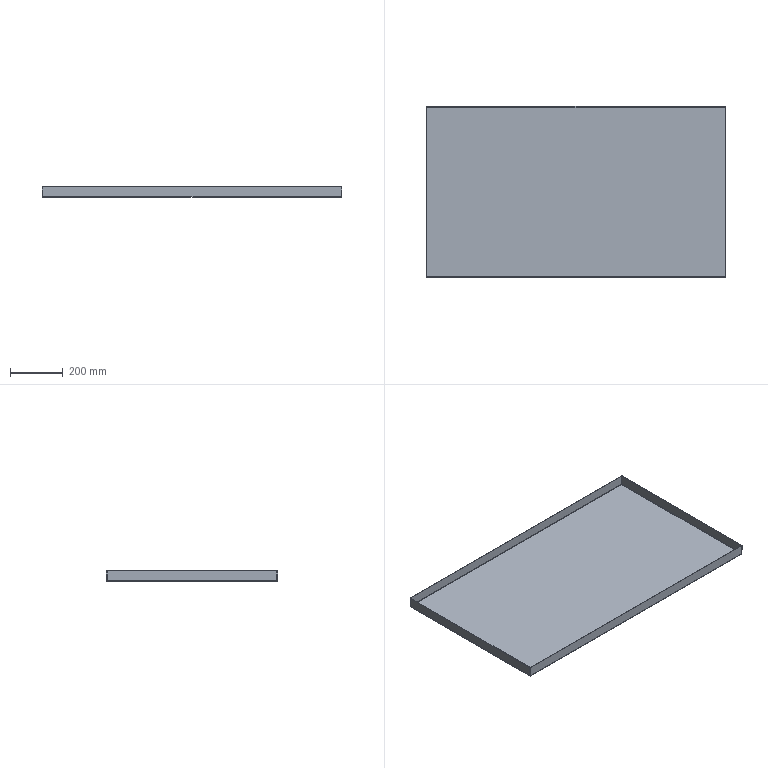Part | SolidWorks | features EdgeFlange 1, FlatPattern 1, SMBaseFlange 1, SheetMetal 1 | 1 solid | 38 faces | box 1140 x 650 x 40 mm | volume 1747070 mm3 | plane 22 | spline 8 | cylinder 8 | commonest cylinder face diameters 1.473 x4 5.473 x4
STEP:
#1=CARTESIAN_POINT('',(567.263,322.263,-2.));
#2=VERTEX_POINT('',#1);
#3=CARTESIAN_POINT('',(567.263,-322.263,-2.));
#4=VERTEX_POINT('',#3);
#5=CARTESIAN_POINT('',(567.263,322.293,-2.));
#6=DIRECTION('',(0.,-1.,0.));
#7=VECTOR('',#6,1000.);
#8=LINE('',#5,#7);
#9=EDGE_CURVE('',#2,#4,#8,.T.);
#10=ORIENTED_EDGE('',*,*,#9,.T.);
#11=CARTESIAN_POINT('',(-567.263,-322.263,-2.));
#12=VERTEX_POINT('',#11);
#13=CARTESIAN_POINT('',(567.293,-322.263,-2.));
#14=DIRECTION('',(-1.,0.,0.));
#15=VECTOR('',#14,1000.);
#16=LINE('',#13,#15);
#17=EDGE_CURVE('',#4,#12,#16,.T.);
#18=ORIENTED_EDGE('',*,*,#17,.T.);
#19=CARTESIAN_POINT('',(-567.263,322.263,-2.));
#20=VERTEX_POINT('',#19);
#21=CARTESIAN_POINT('',(-567.263,-322.293,-2.));
#22=DIRECTION('',(0.,1.,0.));
#23=VECTOR('',#22,1000.);
#24=LINE('',#21,#23);
#25=EDGE_CURVE('',#12,#20,#24,.T.);
#26=ORIENTED_EDGE('',*,*,#25,.T.);
#27=CARTESIAN_POINT('',(-567.293,322.263,-2.));
#28=DIRECTION('',(1.,0.,0.));
#29=VECTOR('',#28,1000.);
#30=LINE('',#27,#29);
#31=EDGE_CURVE('',#20,#2,#30,.T.);
#32=ORIENTED_EDGE('',*,*,#31,.T.);
#33=EDGE_LOOP('',(#10,#18,#26,#32));
#34=FACE_OUTER_BOUND('',#33,.T.);
#35=CARTESIAN_POINT('',(0.,0.,-2.));
#36=DIRECTION('',(0.,0.,-1.));
#37=DIRECTION('',(-1.,0.,0.));
#38=AXIS2_PLACEMENT_3D('',#35,#36,#37);
#39=PLANE('',#38);
#40=ADVANCED_FACE('',(#34),#39,.T.);
#41=CARTESIAN_POINT('',(567.263,-322.263,0.));
#42=VERTEX_POINT('',#41);
#43=CARTESIAN_POINT('',(-567.263,-322.263,0.));
#44=VERTEX_POINT('',#43);
#45=CARTESIAN_POINT('',(567.293,-322.263,0.));
#46=DIRECTION('',(-1.,0.,0.));
#47=VECTOR('',#46,1000.);
#48=LINE('',#45,#47);
#49=EDGE_CURVE('',#42,#44,#48,.T.);
#50=ORIENTED_EDGE('',*,*,#49,.F.);
#51=CARTESIAN_POINT('',(567.263,322.263,0.));
#52=VERTEX_POINT('',#51);
#53=CARTESIAN_POINT('',(567.263,322.293,0.));
#54=DIRECTION('',(0.,-1.,0.));
#55=VECTOR('',#54,1000.);
#56=LINE('',#53,#55);
#57=EDGE_CURVE('',#52,#42,#56,.T.);
#58=ORIENTED_EDGE('',*,*,#57,.F.);
#59=CARTESIAN_POINT('',(-567.263,322.263,0.));
#60=VERTEX_POINT('',#59);
#61=CARTESIAN_POINT('',(-567.293,322.263,0.));
#62=DIRECTION('',(1.,0.,0.));
#63=VECTOR('',#62,1000.);
#64=LINE('',#61,#63);
#65=EDGE_CURVE('',#60,#52,#64,.T.);
#66=ORIENTED_EDGE('',*,*,#65,.F.);
#67=CARTESIAN_POINT('',(-567.263,-322.293,0.));
#68=DIRECTION('',(0.,1.,0.));
#69=VECTOR('',#68,1000.);
#70=LINE('',#67,#69);
#71=EDGE_CURVE('',#44,#60,#70,.T.);
#72=ORIENTED_EDGE('',*,*,#71,.F.);
#73=EDGE_LOOP('',(#50,#58,#66,#72));
#74=FACE_OUTER_BOUND('',#73,.T.);
#75=CARTESIAN_POINT('',(0.,0.,0.));
#76=DIRECTION('',(0.,0.,-1.));
#77=DIRECTION('',(-1.,0.,0.));
#78=AXIS2_PLACEMENT_3D('',#75,#76,#77);
#79=PLANE('',#78);
#80=ADVANCED_FACE('',(#74),#79,.F.);
#81=CARTESIAN_POINT('',(567.293,325.,0.7366));
#82=VERTEX_POINT('',#81);
#83=CARTESIAN_POINT('',(567.293,323.,0.7366));
#84=VERTEX_POINT('',#83);
#85=CARTESIAN_POINT('',(567.293,323.,0.7366));
#86=DIRECTION('',(0.,-1.,0.));
#87=VECTOR('',#86,1000.);
#88=LINE('',#85,#87);
#89=EDGE_CURVE('',#82,#84,#88,.T.);
#90=ORIENTED_EDGE('',*,*,#89,.T.);
#91=CARTESIAN_POINT('',(567.263,322.263,0.));
#92=CARTESIAN_POINT('',(567.268,322.456,0.));
#93=CARTESIAN_POINT('',(567.273,322.648,0.07939));
#94=CARTESIAN_POINT('',(567.283,322.921,0.3521));
#95=CARTESIAN_POINT('',(567.288,323.,0.5438));
#96=CARTESIAN_POINT('',(567.293,323.,0.7366));
#97=B_SPLINE_CURVE_WITH_KNOTS('',3,(#91,#92,#93,#94,#95,#96),.UNSPECIFIED.,.F.,.F.,(4,2,4),(0.,0.5,1.),.UNSPECIFIED.);
#98=EDGE_CURVE('',#52,#84,#97,.T.);
#99=ORIENTED_EDGE('',*,*,#98,.F.);
#100=CARTESIAN_POINT('',(567.263,322.263,0.));
#101=DIRECTION('',(0.,0.,-1.));
#102=VECTOR('',#101,1000.);
#103=LINE('',#100,#102);
#104=EDGE_CURVE('',#52,#2,#103,.T.);
#105=ORIENTED_EDGE('',*,*,#104,.T.);
#106=CARTESIAN_POINT('',(567.263,322.263,-2.));
#107=CARTESIAN_POINT('',(567.266,322.622,-2.));
#108=CARTESIAN_POINT('',(567.268,322.98,-1.929));
#109=CARTESIAN_POINT('',(567.273,323.642,-1.655));
#110=CARTESIAN_POINT('',(567.276,323.945,-1.452));
#111=CARTESIAN_POINT('',(567.281,324.452,-0.9452));
#112=CARTESIAN_POINT('',(567.283,324.655,-0.6416));
#113=CARTESIAN_POINT('',(567.288,324.929,0.0203));
#114=CARTESIAN_POINT('',(567.29,325.,0.3784));
#115=CARTESIAN_POINT('',(567.293,325.,0.7366));
#116=B_SPLINE_CURVE_WITH_KNOTS('',3,(#106,#107,#108,#109,#110,#111,#112,#113,#114,#115),.UNSPECIFIED.,.F.,.F.,(4,2,2,2,4),(0.,0.25,0.5,0.75,1.),.UNSPECIFIED.);
#117=EDGE_CURVE('',#2,#82,#116,.T.);
#118=ORIENTED_EDGE('',*,*,#117,.T.);
#119=EDGE_LOOP('',(#90,#99,#105,#118));
#120=FACE_OUTER_BOUND('',#119,.T.);
#121=CARTESIAN_POINT('',(567.263,322.263,-2.02));
#122=CARTESIAN_POINT('',(567.266,322.624,-2.02));
#123=CARTESIAN_POINT('',(567.268,322.985,-1.948));
#124=CARTESIAN_POINT('',(567.273,323.652,-1.672));
#125=CARTESIAN_POINT('',(567.276,323.957,-1.468));
#126=CARTESIAN_POINT('',(567.281,324.468,-0.9575));
#127=CARTESIAN_POINT('',(567.283,324.672,-0.6517));
#128=CARTESIAN_POINT('',(567.288,324.948,0.01507));
#129=CARTESIAN_POINT('',(567.29,325.02,0.3757));
#130=CARTESIAN_POINT('',(567.293,325.02,0.7366));
#131=CARTESIAN_POINT('',(567.263,322.263,-2.));
#132=CARTESIAN_POINT('',(567.266,322.622,-2.));
#133=CARTESIAN_POINT('',(567.268,322.98,-1.929));
#134=CARTESIAN_POINT('',(567.273,323.642,-1.655));
#135=CARTESIAN_POINT('',(567.276,323.945,-1.452));
#136=CARTESIAN_POINT('',(567.281,324.452,-0.9452));
#137=CARTESIAN_POINT('',(567.283,324.655,-0.6416));
#138=CARTESIAN_POINT('',(567.288,324.929,0.0203));
#139=CARTESIAN_POINT('',(567.29,325.,0.3783));
#140=CARTESIAN_POINT('',(567.293,325.,0.7366));
#141=CARTESIAN_POINT('',(567.263,322.263,0.));
#142=CARTESIAN_POINT('',(567.266,322.36,0.));
#143=CARTESIAN_POINT('',(567.268,322.456,0.01917));
#144=CARTESIAN_POINT('',(567.273,322.634,0.09297));
#145=CARTESIAN_POINT('',(567.276,322.716,0.1476));
#146=CARTESIAN_POINT('',(567.281,322.852,0.2839));
#147=CARTESIAN_POINT('',(567.283,322.907,0.3656));
#148=CARTESIAN_POINT('',(567.288,322.981,0.5438));
#149=CARTESIAN_POINT('',(567.29,323.,0.6402));
#150=CARTESIAN_POINT('',(567.293,323.,0.7366));
#151=CARTESIAN_POINT('',(567.263,322.263,0.0202));
#152=CARTESIAN_POINT('',(567.266,322.357,0.0202));
#153=CARTESIAN_POINT('',(567.268,322.451,0.03885));
#154=CARTESIAN_POINT('',(567.273,322.624,0.1106));
#155=CARTESIAN_POINT('',(567.276,322.704,0.1637));
#156=CARTESIAN_POINT('',(567.281,322.836,0.2963));
#157=CARTESIAN_POINT('',(567.283,322.889,0.3758));
#158=CARTESIAN_POINT('',(567.288,322.961,0.5491));
#159=CARTESIAN_POINT('',(567.29,322.98,0.6428));
#160=CARTESIAN_POINT('',(567.293,322.98,0.7366));
#161=B_SPLINE_SURFACE_WITH_KNOTS('',1,3,((#121,#122,#123,#124,#125,#126,#127,#128,#129,#130),(#131,#132,#133,#134,#135,#136,#137,#138,#139,#140),(#141,#142,#143,#144,#145,#146,#147,#148,#149,#150),(#151,#152,#153,#154,#155,#156,#157,#158,#159,#160)),.UNSPECIFIED.,.F.,.F.,.F.,(2,1,1,2),(4,2,2,2,4),(-0.01,0.,1.,1.01),(0.,0.25,0.5,0.75,1.),.UNSPECIFIED.);
#162=ADVANCED_FACE('',(#120),#161,.F.);
#163=CARTESIAN_POINT('',(-567.293,323.,0.7366));
#164=VERTEX_POINT('',#163);
#165=CARTESIAN_POINT('',(-567.293,323.,0.7366));
#166=CARTESIAN_POINT('',(-567.288,323.,0.5438));
#167=CARTESIAN_POINT('',(-567.283,322.921,0.3521));
#168=CARTESIAN_POINT('',(-567.273,322.648,0.07939));
#169=CARTESIAN_POINT('',(-567.268,322.456,0.));
#170=CARTESIAN_POINT('',(-567.263,322.263,0.));
#171=B_SPLINE_CURVE_WITH_KNOTS('',3,(#165,#166,#167,#168,#169,#170),.UNSPECIFIED.,.F.,.F.,(4,2,4),(0.,0.5,1.),.UNSPECIFIED.);
#172=EDGE_CURVE('',#164,#60,#171,.T.);
#173=ORIENTED_EDGE('',*,*,#172,.F.);
#174=CARTESIAN_POINT('',(-567.293,325.,0.7366));
#175=VERTEX_POINT('',#174);
#176=CARTESIAN_POINT('',(-567.293,323.,0.7366));
#177=DIRECTION('',(0.,-1.,0.));
#178=VECTOR('',#177,1000.);
#179=LINE('',#176,#178);
#180=EDGE_CURVE('',#175,#164,#179,.T.);
#181=ORIENTED_EDGE('',*,*,#180,.F.);
#182=CARTESIAN_POINT('',(-567.293,325.,0.7366));
#183=CARTESIAN_POINT('',(-567.29,325.,0.3784));
#184=CARTESIAN_POINT('',(-567.288,324.929,0.0203));
#185=CARTESIAN_POINT('',(-567.283,324.655,-0.6416));
#186=CARTESIAN_POINT('',(-567.281,324.452,-0.9452));
#187=CARTESIAN_POINT('',(-567.276,323.945,-1.452));
#188=CARTESIAN_POINT('',(-567.273,323.642,-1.655));
#189=CARTESIAN_POINT('',(-567.268,322.98,-1.929));
#190=CARTESIAN_POINT('',(-567.266,322.622,-2.));
#191=CARTESIAN_POINT('',(-567.263,322.263,-2.));
#192=B_SPLINE_CURVE_WITH_KNOTS('',3,(#182,#183,#184,#185,#186,#187,#188,#189,#190,#191),.UNSPECIFIED.,.F.,.F.,(4,2,2,2,4),(0.,0.25,0.5,0.75,1.),.UNSPECIFIED.);
#193=EDGE_CURVE('',#175,#20,#192,.T.);
#194=ORIENTED_EDGE('',*,*,#193,.T.);
#195=CARTESIAN_POINT('',(-567.263,322.263,0.));
#196=DIRECTION('',(0.,0.,-1.));
#197=VECTOR('',#196,1000.);
#198=LINE('',#195,#197);
#199=EDGE_CURVE('',#60,#20,#198,.T.);
#200=ORIENTED_EDGE('',*,*,#199,.F.);
#201=EDGE_LOOP('',(#173,#181,#194,#200));
#202=FACE_OUTER_BOUND('',#201,.T.);
#203=CARTESIAN_POINT('',(-567.293,325.02,0.7366));
#204=CARTESIAN_POINT('',(-567.29,325.02,0.3757));
#205=CARTESIAN_POINT('',(-567.288,324.948,0.01507));
#206=CARTESIAN_POINT('',(-567.283,324.672,-0.6517));
#207=CARTESIAN_POINT('',(-567.281,324.468,-0.9575));
#208=CARTESIAN_POINT('',(-567.276,323.957,-1.468));
#209=CARTESIAN_POINT('',(-567.273,323.652,-1.672));
#210=CARTESIAN_POINT('',(-567.268,322.985,-1.948));
#211=CARTESIAN_POINT('',(-567.266,322.624,-2.02));
#212=CARTESIAN_POINT('',(-567.263,322.263,-2.02));
#213=CARTESIAN_POINT('',(-567.293,325.,0.7366));
#214=CARTESIAN_POINT('',(-567.29,325.,0.3783));
#215=CARTESIAN_POINT('',(-567.288,324.929,0.0203));
#216=CARTESIAN_POINT('',(-567.283,324.655,-0.6416));
#217=CARTESIAN_POINT('',(-567.281,324.452,-0.9452));
#218=CARTESIAN_POINT('',(-567.276,323.945,-1.452));
#219=CARTESIAN_POINT('',(-567.273,323.642,-1.655));
#220=CARTESIAN_POINT('',(-567.268,322.98,-1.929));
#221=CARTESIAN_POINT('',(-567.266,322.622,-2.));
#222=CARTESIAN_POINT('',(-567.263,322.263,-2.));
#223=CARTESIAN_POINT('',(-567.293,323.,0.7366));
#224=CARTESIAN_POINT('',(-567.29,323.,0.6402));
#225=CARTESIAN_POINT('',(-567.288,322.981,0.5438));
#226=CARTESIAN_POINT('',(-567.283,322.907,0.3656));
#227=CARTESIAN_POINT('',(-567.281,322.852,0.2839));
#228=CARTESIAN_POINT('',(-567.276,322.716,0.1476));
#229=CARTESIAN_POINT('',(-567.273,322.634,0.09297));
#230=CARTESIAN_POINT('',(-567.268,322.456,0.01917));
#231=CARTESIAN_POINT('',(-567.266,322.36,0.));
#232=CARTESIAN_POINT('',(-567.263,322.263,0.));
#233=CARTESIAN_POINT('',(-567.293,322.98,0.7366));
#234=CARTESIAN_POINT('',(-567.29,322.98,0.6428));
#235=CARTESIAN_POINT('',(-567.288,322.961,0.5491));
#236=CARTESIAN_POINT('',(-567.283,322.889,0.3758));
#237=CARTESIAN_POINT('',(-567.281,322.836,0.2963));
#238=CARTESIAN_POINT('',(-567.276,322.704,0.1637));
#239=CARTESIAN_POINT('',(-567.273,322.624,0.1106));
#240=CARTESIAN_POINT('',(-567.268,322.451,0.03885));
#241=CARTESIAN_POINT('',(-567.266,322.357,0.0202));
#242=CARTESIAN_POINT('',(-567.263,322.263,0.0202));
#243=B_SPLINE_SURFACE_WITH_KNOTS('',1,3,((#203,#204,#205,#206,#207,#208,#209,#210,#211,#212),(#213,#214,#215,#216,#217,#218,#219,#220,#221,#222),(#223,#224,#225,#226,#227,#228,#229,#230,#231,#232),(#233,#234,#235,#236,#237,#238,#239,#240,#241,#242)),.UNSPECIFIED.,.F.,.F.,.F.,(2,1,1,2),(4,2,2,2,4),(-0.01,0.,1.,1.01),(0.,0.25,0.5,0.75,1.),.UNSPECIFIED.);
#244=ADVANCED_FACE('',(#202),#243,.F.);
#245=ORIENTED_EDGE('',*,*,#31,.F.);
#246=ORIENTED_EDGE('',*,*,#193,.F.);
#247=CARTESIAN_POINT('',(0.,325.,0.7366));
#248=DIRECTION('',(-1.,0.,0.));
#249=VECTOR('',#248,1000.);
#250=LINE('',#247,#249);
#251=EDGE_CURVE('',#82,#175,#250,.T.);
#252=ORIENTED_EDGE('',*,*,#251,.F.);
#253=ORIENTED_EDGE('',*,*,#117,.F.);
#254=EDGE_LOOP('',(#245,#246,#252,#253));
#255=FACE_OUTER_BOUND('',#254,.T.);
#256=CARTESIAN_POINT('',(-567.293,322.263,0.7366));
#257=DIRECTION('',(-1.,0.,0.));
#258=DIRECTION('',(0.,1.,0.));
#259=AXIS2_PLACEMENT_3D('',#256,#257,#258);
#260=CYLINDRICAL_SURFACE('',#259,2.737);
#261=ADVANCED_FACE('',(#255),#260,.T.);
#262=ORIENTED_EDGE('',*,*,#65,.T.);
#263=ORIENTED_EDGE('',*,*,#98,.T.);
#264=CARTESIAN_POINT('',(570.,323.,0.7366));
#265=DIRECTION('',(-1.,0.,0.));
#266=VECTOR('',#265,1000.);
#267=LINE('',#264,#266);
#268=EDGE_CURVE('',#84,#164,#267,.T.);
#269=ORIENTED_EDGE('',*,*,#268,.T.);
#270=ORIENTED_EDGE('',*,*,#172,.T.);
#271=EDGE_LOOP('',(#262,#263,#269,#270));
#272=FACE_OUTER_BOUND('',#271,.T.);
#273=CARTESIAN_POINT('',(-567.293,322.263,0.7366));
#274=DIRECTION('',(-1.,0.,0.));
#275=DIRECTION('',(0.,1.,0.));
#276=AXIS2_PLACEMENT_3D('',#273,#274,#275);
#277=CYLINDRICAL_SURFACE('',#276,0.7366);
#278=ADVANCED_FACE('',(#272),#277,.F.);
#279=CARTESIAN_POINT('',(567.293,323.,38.));
#280=VERTEX_POINT('',#279);
#281=CARTESIAN_POINT('',(567.293,325.,38.));
#282=VERTEX_POINT('',#281);
#283=CARTESIAN_POINT('',(567.293,325.,38.));
#284=DIRECTION('',(0.,1.,0.));
#285=VECTOR('',#284,1000.);
#286=LINE('',#283,#285);
#287=EDGE_CURVE('',#280,#282,#286,.T.);
#288=ORIENTED_EDGE('',*,*,#287,.F.);
#289=CARTESIAN_POINT('',(567.293,323.,0.));
#290=DIRECTION('',(0.,0.,1.));
#291=VECTOR('',#290,1000.);
#292=LINE('',#289,#291);
#293=EDGE_CURVE('',#84,#280,#292,.T.);
#294=ORIENTED_EDGE('',*,*,#293,.F.);
#295=ORIENTED_EDGE('',*,*,#89,.F.);
#296=CARTESIAN_POINT('',(567.293,325.,0.));
#297=DIRECTION('',(0.,0.,-1.));
#298=VECTOR('',#297,1000.);
#299=LINE('',#296,#298);
#300=EDGE_CURVE('',#282,#82,#299,.T.);
#301=ORIENTED_EDGE('',*,*,#300,.F.);
#302=EDGE_LOOP('',(#288,#294,#295,#301));
#303=FACE_OUTER_BOUND('',#302,.T.);
#304=CARTESIAN_POINT('',(567.293,323.,0.));
#305=DIRECTION('',(1.,0.,0.));
#306=DIRECTION('',(0.,0.,-1.));
#307=AXIS2_PLACEMENT_3D('',#304,#305,#306);
#308=PLANE('',#307);
#309=ADVANCED_FACE('',(#303),#308,.T.);
#310=CARTESIAN_POINT('',(-567.293,325.,38.));
#311=VERTEX_POINT('',#310);
#312=CARTESIAN_POINT('',(-567.293,325.,0.));
#313=DIRECTION('',(0.,0.,-1.));
#314=VECTOR('',#313,1000.);
#315=LINE('',#312,#314);
#316=EDGE_CURVE('',#311,#175,#315,.T.);
#317=ORIENTED_EDGE('',*,*,#316,.F.);
#318=CARTESIAN_POINT('',(-570.,325.,38.));
#319=DIRECTION('',(-1.,0.,0.));
#320=VECTOR('',#319,1000.);
#321=LINE('',#318,#320);
#322=EDGE_CURVE('',#282,#311,#321,.T.);
#323=ORIENTED_EDGE('',*,*,#322,.F.);
#324=ORIENTED_EDGE('',*,*,#300,.T.);
#325=ORIENTED_EDGE('',*,*,#251,.T.);
#326=EDGE_LOOP('',(#317,#323,#324,#325));
#327=FACE_OUTER_BOUND('',#326,.T.);
#328=CARTESIAN_POINT('',(0.,325.,0.));
#329=DIRECTION('',(0.,1.,0.));
#330=DIRECTION('',(0.,0.,1.));
#331=AXIS2_PLACEMENT_3D('',#328,#329,#330);
#332=PLANE('',#331);
#333=ADVANCED_FACE('',(#327),#332,.T.);
#334=CARTESIAN_POINT('',(-567.293,323.,38.));
#335=VERTEX_POINT('',#334);
#336=CARTESIAN_POINT('',(0.,323.,38.));
#337=DIRECTION('',(-1.,0.,0.));
#338=VECTOR('',#337,1000.);
#339=LINE('',#336,#338);
#340=EDGE_CURVE('',#280,#335,#339,.T.);
#341=ORIENTED_EDGE('',*,*,#340,.T.);
#342=CARTESIAN_POINT('',(-567.293,323.,0.));
#343=DIRECTION('',(0.,0.,1.));
#344=VECTOR('',#343,1000.);
#345=LINE('',#342,#344);
#346=EDGE_CURVE('',#164,#335,#345,.T.);
#347=ORIENTED_EDGE('',*,*,#346,.F.);
#348=ORIENTED_EDGE('',*,*,#268,.F.);
#349=ORIENTED_EDGE('',*,*,#293,.T.);
#350=EDGE_LOOP('',(#341,#347,#348,#349));
#351=FACE_OUTER_BOUND('',#350,.T.);
#352=CARTESIAN_POINT('',(0.,323.,0.));
#353=DIRECTION('',(0.,1.,0.));
#354=DIRECTION('',(0.,0.,1.));
#355=AXIS2_PLACEMENT_3D('',#352,#353,#354);
#356=PLANE('',#355);
#357=ADVANCED_FACE('',(#351),#356,.F.);
#358=CARTESIAN_POINT('',(-567.293,323.,38.));
#359=DIRECTION('',(0.,1.,0.));
#360=VECTOR('',#359,1000.);
#361=LINE('',#358,#360);
#362=EDGE_CURVE('',#335,#311,#361,.T.);
#363=ORIENTED_EDGE('',*,*,#362,.F.);
#364=ORIENTED_EDGE('',*,*,#340,.F.);
#365=ORIENTED_EDGE('',*,*,#287,.T.);
#366=ORIENTED_EDGE('',*,*,#322,.T.);
#367=EDGE_LOOP('',(#363,#364,#365,#366));
#368=FACE_OUTER_BOUND('',#367,.T.);
#369=CARTESIAN_POINT('',(-570.,325.,38.));
#370=DIRECTION('',(0.,0.,1.));
#371=DIRECTION('',(0.,-1.,0.));
#372=AXIS2_PLACEMENT_3D('',#369,#370,#371);
#373=PLANE('',#372);
#374=ADVANCED_FACE('',(#368),#373,.T.);
#375=ORIENTED_EDGE('',*,*,#346,.T.);
#376=ORIENTED_EDGE('',*,*,#362,.T.);
#377=ORIENTED_EDGE('',*,*,#316,.T.);
#378=ORIENTED_EDGE('',*,*,#180,.T.);
#379=EDGE_LOOP('',(#375,#376,#377,#378));
#380=FACE_OUTER_BOUND('',#379,.T.);
#381=CARTESIAN_POINT('',(-567.293,323.,0.));
#382=DIRECTION('',(1.,0.,0.));
#383=DIRECTION('',(0.,0.,-1.));
#384=AXIS2_PLACEMENT_3D('',#381,#382,#383);
#385=PLANE('',#384);
#386=ADVANCED_FACE('',(#380),#385,.F.);
#387=CARTESIAN_POINT('',(-570.,322.293,0.7366));
#388=VERTEX_POINT('',#387);
#389=CARTESIAN_POINT('',(-568.,322.293,0.7366));
#390=VERTEX_POINT('',#389);
#391=CARTESIAN_POINT('',(-568.,322.293,0.7366));
#392=DIRECTION('',(1.,0.,0.));
#393=VECTOR('',#392,1000.);
#394=LINE('',#391,#393);
#395=EDGE_CURVE('',#388,#390,#394,.T.);
#396=ORIENTED_EDGE('',*,*,#395,.T.);
#397=CARTESIAN_POINT('',(-567.263,322.263,0.));
#398=CARTESIAN_POINT('',(-567.456,322.268,0.));
#399=CARTESIAN_POINT('',(-567.648,322.273,0.07939));
#400=CARTESIAN_POINT('',(-567.921,322.283,0.3521));
#401=CARTESIAN_POINT('',(-568.,322.288,0.5438));
#402=CARTESIAN_POINT('',(-568.,322.293,0.7366));
#403=B_SPLINE_CURVE_WITH_KNOTS('',3,(#397,#398,#399,#400,#401,#402),.UNSPECIFIED.,.F.,.F.,(4,2,4),(0.,0.5,1.),.UNSPECIFIED.);
#404=EDGE_CURVE('',#60,#390,#403,.T.);
#405=ORIENTED_EDGE('',*,*,#404,.F.);
#406=ORIENTED_EDGE('',*,*,#199,.T.);
#407=CARTESIAN_POINT('',(-567.263,322.263,-2.));
#408=CARTESIAN_POINT('',(-567.622,322.266,-2.));
#409=CARTESIAN_POINT('',(-567.98,322.268,-1.929));
#410=CARTESIAN_POINT('',(-568.642,322.273,-1.655));
#411=CARTESIAN_POINT('',(-568.945,322.276,-1.452));
#412=CARTESIAN_POINT('',(-569.452,322.281,-0.9452));
#413=CARTESIAN_POINT('',(-569.655,322.283,-0.6416));
#414=CARTESIAN_POINT('',(-569.929,322.288,0.0203));
#415=CARTESIAN_POINT('',(-570.,322.29,0.3784));
#416=CARTESIAN_POINT('',(-570.,322.293,0.7366));
#417=B_SPLINE_CURVE_WITH_KNOTS('',3,(#407,#408,#409,#410,#411,#412,#413,#414,#415,#416),.UNSPECIFIED.,.F.,.F.,(4,2,2,2,4),(0.,0.25,0.5,0.75,1.),.UNSPECIFIED.);
#418=EDGE_CURVE('',#20,#388,#417,.T.);
#419=ORIENTED_EDGE('',*,*,#418,.T.);
#420=EDGE_LOOP('',(#396,#405,#406,#419));
#421=FACE_OUTER_BOUND('',#420,.T.);
#422=CARTESIAN_POINT('',(-567.263,322.263,-2.02));
#423=CARTESIAN_POINT('',(-567.624,322.266,-2.02));
#424=CARTESIAN_POINT('',(-567.985,322.268,-1.948));
#425=CARTESIAN_POINT('',(-568.652,322.273,-1.672));
#426=CARTESIAN_POINT('',(-568.957,322.276,-1.468));
#427=CARTESIAN_POINT('',(-569.468,322.281,-0.9575));
#428=CARTESIAN_POINT('',(-569.672,322.283,-0.6517));
#429=CARTESIAN_POINT('',(-569.948,322.288,0.01507));
#430=CARTESIAN_POINT('',(-570.02,322.29,0.3757));
#431=CARTESIAN_POINT('',(-570.02,322.293,0.7366));
#432=CARTESIAN_POINT('',(-567.263,322.263,-2.));
#433=CARTESIAN_POINT('',(-567.622,322.266,-2.));
#434=CARTESIAN_POINT('',(-567.98,322.268,-1.929));
#435=CARTESIAN_POINT('',(-568.642,322.273,-1.655));
#436=CARTESIAN_POINT('',(-568.945,322.276,-1.452));
#437=CARTESIAN_POINT('',(-569.452,322.281,-0.9452));
#438=CARTESIAN_POINT('',(-569.655,322.283,-0.6416));
#439=CARTESIAN_POINT('',(-569.929,322.288,0.0203));
#440=CARTESIAN_POINT('',(-570.,322.29,0.3783));
#441=CARTESIAN_POINT('',(-570.,322.293,0.7366));
#442=CARTESIAN_POINT('',(-567.263,322.263,0.));
#443=CARTESIAN_POINT('',(-567.36,322.266,0.));
#444=CARTESIAN_POINT('',(-567.456,322.268,0.01917));
#445=CARTESIAN_POINT('',(-567.634,322.273,0.09297));
#446=CARTESIAN_POINT('',(-567.716,322.276,0.1476));
#447=CARTESIAN_POINT('',(-567.852,322.281,0.2839));
#448=CARTESIAN_POINT('',(-567.907,322.283,0.3656));
#449=CARTESIAN_POINT('',(-567.981,322.288,0.5438));
#450=CARTESIAN_POINT('',(-568.,322.29,0.6402));
#451=CARTESIAN_POINT('',(-568.,322.293,0.7366));
#452=CARTESIAN_POINT('',(-567.263,322.263,0.0202));
#453=CARTESIAN_POINT('',(-567.357,322.266,0.0202));
#454=CARTESIAN_POINT('',(-567.451,322.268,0.03885));
#455=CARTESIAN_POINT('',(-567.624,322.273,0.1106));
#456=CARTESIAN_POINT('',(-567.704,322.276,0.1637));
#457=CARTESIAN_POINT('',(-567.836,322.281,0.2963));
#458=CARTESIAN_POINT('',(-567.889,322.283,0.3758));
#459=CARTESIAN_POINT('',(-567.961,322.288,0.5491));
#460=CARTESIAN_POINT('',(-567.98,322.29,0.6428));
#461=CARTESIAN_POINT('',(-567.98,322.293,0.7366));
#462=B_SPLINE_SURFACE_WITH_KNOTS('',1,3,((#422,#423,#424,#425,#426,#427,#428,#429,#430,#431),(#432,#433,#434,#435,#436,#437,#438,#439,#440,#441),(#442,#443,#444,#445,#446,#447,#448,#449,#450,#451),(#452,#453,#454,#455,#456,#457,#458,#459,#460,#461)),.UNSPECIFIED.,.F.,.F.,.F.,(2,1,1,2),(4,2,2,2,4),(-0.01,0.,1.,1.01),(0.,0.25,0.5,0.75,1.),.UNSPECIFIED.);
#463=ADVANCED_FACE('',(#421),#462,.F.);
#464=CARTESIAN_POINT('',(-568.,-322.293,0.7366));
#465=VERTEX_POINT('',#464);
#466=CARTESIAN_POINT('',(-568.,-322.293,0.7366));
#467=CARTESIAN_POINT('',(-568.,-322.288,0.5438));
#468=CARTESIAN_POINT('',(-567.921,-322.283,0.3521));
#469=CARTESIAN_POINT('',(-567.648,-322.273,0.07939));
#470=CARTESIAN_POINT('',(-567.456,-322.268,0.));
#471=CARTESIAN_POINT('',(-567.263,-322.263,0.));
#472=B_SPLINE_CURVE_WITH_KNOTS('',3,(#466,#467,#468,#469,#470,#471),.UNSPECIFIED.,.F.,.F.,(4,2,4),(0.,0.5,1.),.UNSPECIFIED.);
#473=EDGE_CURVE('',#465,#44,#472,.T.);
#474=ORIENTED_EDGE('',*,*,#473,.F.);
#475=CARTESIAN_POINT('',(-570.,-322.293,0.7366));
#476=VERTEX_POINT('',#475);
#477=CARTESIAN_POINT('',(-568.,-322.293,0.7366));
#478=DIRECTION('',(1.,0.,0.));
#479=VECTOR('',#478,1000.);
#480=LINE('',#477,#479);
#481=EDGE_CURVE('',#476,#465,#480,.T.);
#482=ORIENTED_EDGE('',*,*,#481,.F.);
#483=CARTESIAN_POINT('',(-570.,-322.293,0.7366));
#484=CARTESIAN_POINT('',(-570.,-322.29,0.3784));
#485=CARTESIAN_POINT('',(-569.929,-322.288,0.0203));
#486=CARTESIAN_POINT('',(-569.655,-322.283,-0.6416));
#487=CARTESIAN_POINT('',(-569.452,-322.281,-0.9452));
#488=CARTESIAN_POINT('',(-568.945,-322.276,-1.452));
#489=CARTESIAN_POINT('',(-568.642,-322.273,-1.655));
#490=CARTESIAN_POINT('',(-567.98,-322.268,-1.929));
#491=CARTESIAN_POINT('',(-567.622,-322.266,-2.));
#492=CARTESIAN_POINT('',(-567.263,-322.263,-2.));
#493=B_SPLINE_CURVE_WITH_KNOTS('',3,(#483,#484,#485,#486,#487,#488,#489,#490,#491,#492),.UNSPECIFIED.,.F.,.F.,(4,2,2,2,4),(0.,0.25,0.5,0.75,1.),.UNSPECIFIED.);
#494=EDGE_CURVE('',#476,#12,#493,.T.);
#495=ORIENTED_EDGE('',*,*,#494,.T.);
#496=CARTESIAN_POINT('',(-567.263,-322.263,0.));
#497=DIRECTION('',(0.,0.,-1.));
#498=VECTOR('',#497,1000.);
#499=LINE('',#496,#498);
#500=EDGE_CURVE('',#44,#12,#499,.T.);
#501=ORIENTED_EDGE('',*,*,#500,.F.);
#502=EDGE_LOOP('',(#474,#482,#495,#501));
#503=FACE_OUTER_BOUND('',#502,.T.);
#504=CARTESIAN_POINT('',(-570.02,-322.293,0.7366));
#505=CARTESIAN_POINT('',(-570.02,-322.29,0.3757));
#506=CARTESIAN_POINT('',(-569.948,-322.288,0.01507));
#507=CARTESIAN_POINT('',(-569.672,-322.283,-0.6517));
#508=CARTESIAN_POINT('',(-569.468,-322.281,-0.9575));
#509=CARTESIAN_POINT('',(-568.957,-322.276,-1.468));
#510=CARTESIAN_POINT('',(-568.652,-322.273,-1.672));
#511=CARTESIAN_POINT('',(-567.985,-322.268,-1.948));
#512=CARTESIAN_POINT('',(-567.624,-322.266,-2.02));
#513=CARTESIAN_POINT('',(-567.263,-322.263,-2.02));
#514=CARTESIAN_POINT('',(-570.,-322.293,0.7366));
#515=CARTESIAN_POINT('',(-570.,-322.29,0.3783));
#516=CARTESIAN_POINT('',(-569.929,-322.288,0.0203));
#517=CARTESIAN_POINT('',(-569.655,-322.283,-0.6416));
#518=CARTESIAN_POINT('',(-569.452,-322.281,-0.9452));
#519=CARTESIAN_POINT('',(-568.945,-322.276,-1.452));
#520=CARTESIAN_POINT('',(-568.642,-322.273,-1.655));
#521=CARTESIAN_POINT('',(-567.98,-322.268,-1.929));
#522=CARTESIAN_POINT('',(-567.622,-322.266,-2.));
#523=CARTESIAN_POINT('',(-567.263,-322.263,-2.));
#524=CARTESIAN_POINT('',(-568.,-322.293,0.7366));
#525=CARTESIAN_POINT('',(-568.,-322.29,0.6402));
#526=CARTESIAN_POINT('',(-567.981,-322.288,0.5438));
#527=CARTESIAN_POINT('',(-567.907,-322.283,0.3656));
#528=CARTESIAN_POINT('',(-567.852,-322.281,0.2839));
#529=CARTESIAN_POINT('',(-567.716,-322.276,0.1476));
#530=CARTESIAN_POINT('',(-567.634,-322.273,0.09297));
#531=CARTESIAN_POINT('',(-567.456,-322.268,0.01917));
#532=CARTESIAN_POINT('',(-567.36,-322.266,0.));
#533=CARTESIAN_POINT('',(-567.263,-322.263,0.));
#534=CARTESIAN_POINT('',(-567.98,-322.293,0.7366));
#535=CARTESIAN_POINT('',(-567.98,-322.29,0.6428));
#536=CARTESIAN_POINT('',(-567.961,-322.288,0.5491));
#537=CARTESIAN_POINT('',(-567.889,-322.283,0.3758));
#538=CARTESIAN_POINT('',(-567.836,-322.281,0.2963));
#539=CARTESIAN_POINT('',(-567.704,-322.276,0.1637));
#540=CARTESIAN_POINT('',(-567.624,-322.273,0.1106));
#541=CARTESIAN_POINT('',(-567.451,-322.268,0.03885));
#542=CARTESIAN_POINT('',(-567.357,-322.266,0.0202));
#543=CARTESIAN_POINT('',(-567.263,-322.263,0.0202));
#544=B_SPLINE_SURFACE_WITH_KNOTS('',1,3,((#504,#505,#506,#507,#508,#509,#510,#511,#512,#513),(#514,#515,#516,#517,#518,#519,#520,#521,#522,#523),(#524,#525,#526,#527,#528,#529,#530,#531,#532,#533),(#534,#535,#536,#537,#538,#539,#540,#541,#542,#543)),.UNSPECIFIED.,.F.,.F.,.F.,(2,1,1,2),(4,2,2,2,4),(-0.01,0.,1.,1.01),(0.,0.25,0.5,0.75,1.),.UNSPECIFIED.);
#545=ADVANCED_FACE('',(#503),#544,.F.);
#546=ORIENTED_EDGE('',*,*,#25,.F.);
#547=ORIENTED_EDGE('',*,*,#494,.F.);
#548=CARTESIAN_POINT('',(-570.,325.,0.7366));
#549=DIRECTION('',(0.,1.,0.));
#550=VECTOR('',#549,1000.);
#551=LINE('',#548,#550);
#552=EDGE_CURVE('',#476,#388,#551,.T.);
#553=ORIENTED_EDGE('',*,*,#552,.T.);
#554=ORIENTED_EDGE('',*,*,#418,.F.);
#555=EDGE_LOOP('',(#546,#547,#553,#554));
#556=FACE_OUTER_BOUND('',#555,.T.);
#557=CARTESIAN_POINT('',(-567.263,-322.293,0.7366));
#558=DIRECTION('',(0.,-1.,0.));
#559=DIRECTION('',(-1.,0.,0.));
#560=AXIS2_PLACEMENT_3D('',#557,#558,#559);
#561=CYLINDRICAL_SURFACE('',#560,2.737);
#562=ADVANCED_FACE('',(#556),#561,.T.);
#563=ORIENTED_EDGE('',*,*,#71,.T.);
#564=ORIENTED_EDGE('',*,*,#404,.T.);
#565=CARTESIAN_POINT('',(-568.,325.,0.7366));
#566=DIRECTION('',(0.,-1.,0.));
#567=VECTOR('',#566,1000.);
#568=LINE('',#565,#567);
#569=EDGE_CURVE('',#390,#465,#568,.T.);
#570=ORIENTED_EDGE('',*,*,#569,.T.);
#571=ORIENTED_EDGE('',*,*,#473,.T.);
#572=EDGE_LOOP('',(#563,#564,#570,#571));
#573=FACE_OUTER_BOUND('',#572,.T.);
#574=CARTESIAN_POINT('',(-567.263,-322.293,0.7366));
#575=DIRECTION('',(0.,-1.,0.));
#576=DIRECTION('',(-1.,0.,0.));
#577=AXIS2_PLACEMENT_3D('',#574,#575,#576);
#578=CYLINDRICAL_SURFACE('',#577,0.7366);
#579=ADVANCED_FACE('',(#573),#578,.F.);
#580=CARTESIAN_POINT('',(-568.,322.293,38.));
#581=VERTEX_POINT('',#580);
#582=CARTESIAN_POINT('',(-570.,322.293,38.));
#583=VERTEX_POINT('',#582);
#584=CARTESIAN_POINT('',(-570.,322.293,38.));
#585=DIRECTION('',(-1.,0.,0.));
#586=VECTOR('',#585,1000.);
#587=LINE('',#584,#586);
#588=EDGE_CURVE('',#581,#583,#587,.T.);
#589=ORIENTED_EDGE('',*,*,#588,.F.);
#590=CARTESIAN_POINT('',(-568.,322.293,0.));
#591=DIRECTION('',(0.,0.,1.));
#592=VECTOR('',#591,1000.);
#593=LINE('',#590,#592);
#594=EDGE_CURVE('',#390,#581,#593,.T.);
#595=ORIENTED_EDGE('',*,*,#594,.F.);
#596=ORIENTED_EDGE('',*,*,#395,.F.);
#597=CARTESIAN_POINT('',(-570.,322.293,0.));
#598=DIRECTION('',(0.,0.,1.));
#599=VECTOR('',#598,1000.);
#600=LINE('',#597,#599);
#601=EDGE_CURVE('',#388,#583,#600,.T.);
#602=ORIENTED_EDGE('',*,*,#601,.T.);
#603=EDGE_LOOP('',(#589,#595,#596,#602));
#604=FACE_OUTER_BOUND('',#603,.T.);
#605=CARTESIAN_POINT('',(-568.,322.293,0.));
#606=DIRECTION('',(0.,1.,0.));
#607=DIRECTION('',(0.,0.,1.));
#608=AXIS2_PLACEMENT_3D('',#605,#606,#607);
#609=PLANE('',#608);
#610=ADVANCED_FACE('',(#604),#609,.T.);
#611=ORIENTED_EDGE('',*,*,#552,.F.);
#612=CARTESIAN_POINT('',(-570.,-322.293,38.));
#613=VERTEX_POINT('',#612);
#614=CARTESIAN_POINT('',(-570.,-322.293,0.));
#615=DIRECTION('',(0.,0.,1.));
#616=VECTOR('',#615,1000.);
#617=LINE('',#614,#616);
#618=EDGE_CURVE('',#476,#613,#617,.T.);
#619=ORIENTED_EDGE('',*,*,#618,.T.);
#620=CARTESIAN_POINT('',(-570.,325.,38.));
#621=DIRECTION('',(0.,-1.,0.));
#622=VECTOR('',#621,1000.);
#623=LINE('',#620,#622);
#624=EDGE_CURVE('',#583,#613,#623,.T.);
#625=ORIENTED_EDGE('',*,*,#624,.F.);
#626=ORIENTED_EDGE('',*,*,#601,.F.);
#627=EDGE_LOOP('',(#611,#619,#625,#626));
#628=FACE_OUTER_BOUND('',#627,.T.);
#629=CARTESIAN_POINT('',(-570.,0.,0.));
#630=DIRECTION('',(1.,0.,0.));
#631=DIRECTION('',(0.,0.,-1.));
#632=AXIS2_PLACEMENT_3D('',#629,#630,#631);
#633=PLANE('',#632);
#634=ADVANCED_FACE('',(#628),#633,.F.);
#635=CARTESIAN_POINT('',(-568.,-322.293,38.));
#636=VERTEX_POINT('',#635);
#637=CARTESIAN_POINT('',(-568.,-322.293,0.));
#638=DIRECTION('',(0.,0.,1.));
#639=VECTOR('',#638,1000.);
#640=LINE('',#637,#639);
#641=EDGE_CURVE('',#465,#636,#640,.T.);
#642=ORIENTED_EDGE('',*,*,#641,.F.);
#643=ORIENTED_EDGE('',*,*,#569,.F.);
#644=ORIENTED_EDGE('',*,*,#594,.T.);
#645=CARTESIAN_POINT('',(-568.,0.,38.));
#646=DIRECTION('',(0.,-1.,0.));
#647=VECTOR('',#646,1000.);
#648=LINE('',#645,#647);
#649=EDGE_CURVE('',#581,#636,#648,.T.);
#650=ORIENTED_EDGE('',*,*,#649,.T.);
#651=EDGE_LOOP('',(#642,#643,#644,#650));
#652=FACE_OUTER_BOUND('',#651,.T.);
#653=CARTESIAN_POINT('',(-568.,0.,0.));
#654=DIRECTION('',(1.,0.,0.));
#655=DIRECTION('',(0.,0.,-1.));
#656=AXIS2_PLACEMENT_3D('',#653,#654,#655);
#657=PLANE('',#656);
#658=ADVANCED_FACE('',(#652),#657,.T.);
#659=CARTESIAN_POINT('',(-568.,-322.293,38.));
#660=DIRECTION('',(-1.,0.,0.));
#661=VECTOR('',#660,1000.);
#662=LINE('',#659,#661);
#663=EDGE_CURVE('',#636,#613,#662,.T.);
#664=ORIENTED_EDGE('',*,*,#663,.F.);
#665=ORIENTED_EDGE('',*,*,#649,.F.);
#666=ORIENTED_EDGE('',*,*,#588,.T.);
#667=ORIENTED_EDGE('',*,*,#624,.T.);
#668=EDGE_LOOP('',(#664,#665,#666,#667));
#669=FACE_OUTER_BOUND('',#668,.T.);
#670=CARTESIAN_POINT('',(-570.,325.,38.));
#671=DIRECTION('',(0.,0.,1.));
#672=DIRECTION('',(1.,0.,0.));
#673=AXIS2_PLACEMENT_3D('',#670,#671,#672);
#674=PLANE('',#673);
#675=ADVANCED_FACE('',(#669),#674,.T.);
#676=ORIENTED_EDGE('',*,*,#641,.T.);
#677=ORIENTED_EDGE('',*,*,#663,.T.);
#678=ORIENTED_EDGE('',*,*,#618,.F.);
#679=ORIENTED_EDGE('',*,*,#481,.T.);
#680=EDGE_LOOP('',(#676,#677,#678,#679));
#681=FACE_OUTER_BOUND('',#680,.T.);
#682=CARTESIAN_POINT('',(-568.,-322.293,0.));
#683=DIRECTION('',(0.,1.,0.));
#684=DIRECTION('',(0.,0.,1.));
#685=AXIS2_PLACEMENT_3D('',#682,#683,#684);
#686=PLANE('',#685);
#687=ADVANCED_FACE('',(#681),#686,.F.);
#688=CARTESIAN_POINT('',(570.,-322.293,0.7366));
#689=VERTEX_POINT('',#688);
#690=CARTESIAN_POINT('',(568.,-322.293,0.7366));
#691=VERTEX_POINT('',#690);
#692=CARTESIAN_POINT('',(568.,-322.293,0.7366));
#693=DIRECTION('',(-1.,0.,0.));
#694=VECTOR('',#693,1000.);
#695=LINE('',#692,#694);
#696=EDGE_CURVE('',#689,#691,#695,.T.);
#697=ORIENTED_EDGE('',*,*,#696,.T.);
#698=CARTESIAN_POINT('',(567.263,-322.263,0.));
#699=CARTESIAN_POINT('',(567.456,-322.268,0.));
#700=CARTESIAN_POINT('',(567.648,-322.273,0.07939));
#701=CARTESIAN_POINT('',(567.921,-322.283,0.3521));
#702=CARTESIAN_POINT('',(568.,-322.288,0.5438));
#703=CARTESIAN_POINT('',(568.,-322.293,0.7366));
#704=B_SPLINE_CURVE_WITH_KNOTS('',3,(#698,#699,#700,#701,#702,#703),.UNSPECIFIED.,.F.,.F.,(4,2,4),(0.,0.5,1.),.UNSPECIFIED.);
#705=EDGE_CURVE('',#42,#691,#704,.T.);
#706=ORIENTED_EDGE('',*,*,#705,.F.);
#707=CARTESIAN_POINT('',(567.263,-322.263,0.));
#708=DIRECTION('',(0.,0.,-1.));
#709=VECTOR('',#708,1000.);
#710=LINE('',#707,#709);
#711=EDGE_CURVE('',#42,#4,#710,.T.);
#712=ORIENTED_EDGE('',*,*,#711,.T.);
#713=CARTESIAN_POINT('',(567.263,-322.263,-2.));
#714=CARTESIAN_POINT('',(567.622,-322.266,-2.));
#715=CARTESIAN_POINT('',(567.98,-322.268,-1.929));
#716=CARTESIAN_POINT('',(568.642,-322.273,-1.655));
#717=CARTESIAN_POINT('',(568.945,-322.276,-1.452));
#718=CARTESIAN_POINT('',(569.452,-322.281,-0.9452));
#719=CARTESIAN_POINT('',(569.655,-322.283,-0.6416));
#720=CARTESIAN_POINT('',(569.929,-322.288,0.0203));
#721=CARTESIAN_POINT('',(570.,-322.29,0.3784));
#722=CARTESIAN_POINT('',(570.,-322.293,0.7366));
#723=B_SPLINE_CURVE_WITH_KNOTS('',3,(#713,#714,#715,#716,#717,#718,#719,#720,#721,#722),.UNSPECIFIED.,.F.,.F.,(4,2,2,2,4),(0.,0.25,0.5,0.75,1.),.UNSPECIFIED.);
#724=EDGE_CURVE('',#4,#689,#723,.T.);
#725=ORIENTED_EDGE('',*,*,#724,.T.);
#726=EDGE_LOOP('',(#697,#706,#712,#725));
#727=FACE_OUTER_BOUND('',#726,.T.);
#728=CARTESIAN_POINT('',(567.263,-322.263,-2.02));
#729=CARTESIAN_POINT('',(567.624,-322.266,-2.02));
#730=CARTESIAN_POINT('',(567.985,-322.268,-1.948));
#731=CARTESIAN_POINT('',(568.652,-322.273,-1.672));
#732=CARTESIAN_POINT('',(568.957,-322.276,-1.468));
#733=CARTESIAN_POINT('',(569.468,-322.281,-0.9575));
#734=CARTESIAN_POINT('',(569.672,-322.283,-0.6517));
#735=CARTESIAN_POINT('',(569.948,-322.288,0.01507));
#736=CARTESIAN_POINT('',(570.02,-322.29,0.3757));
#737=CARTESIAN_POINT('',(570.02,-322.293,0.7366));
#738=CARTESIAN_POINT('',(567.263,-322.263,-2.));
#739=CARTESIAN_POINT('',(567.622,-322.266,-2.));
#740=CARTESIAN_POINT('',(567.98,-322.268,-1.929));
#741=CARTESIAN_POINT('',(568.642,-322.273,-1.655));
#742=CARTESIAN_POINT('',(568.945,-322.276,-1.452));
#743=CARTESIAN_POINT('',(569.452,-322.281,-0.9452));
#744=CARTESIAN_POINT('',(569.655,-322.283,-0.6416));
#745=CARTESIAN_POINT('',(569.929,-322.288,0.0203));
#746=CARTESIAN_POINT('',(570.,-322.29,0.3783));
#747=CARTESIAN_POINT('',(570.,-322.293,0.7366));
#748=CARTESIAN_POINT('',(567.263,-322.263,0.));
#749=CARTESIAN_POINT('',(567.36,-322.266,0.));
#750=CARTESIAN_POINT('',(567.456,-322.268,0.01917));
#751=CARTESIAN_POINT('',(567.634,-322.273,0.09297));
#752=CARTESIAN_POINT('',(567.716,-322.276,0.1476));
#753=CARTESIAN_POINT('',(567.852,-322.281,0.2839));
#754=CARTESIAN_POINT('',(567.907,-322.283,0.3656));
#755=CARTESIAN_POINT('',(567.981,-322.288,0.5438));
#756=CARTESIAN_POINT('',(568.,-322.29,0.6402));
#757=CARTESIAN_POINT('',(568.,-322.293,0.7366));
#758=CARTESIAN_POINT('',(567.263,-322.263,0.0202));
#759=CARTESIAN_POINT('',(567.357,-322.266,0.0202));
#760=CARTESIAN_POINT('',(567.451,-322.268,0.03885));
#761=CARTESIAN_POINT('',(567.624,-322.273,0.1106));
#762=CARTESIAN_POINT('',(567.704,-322.276,0.1637));
#763=CARTESIAN_POINT('',(567.836,-322.281,0.2963));
#764=CARTESIAN_POINT('',(567.889,-322.283,0.3758));
#765=CARTESIAN_POINT('',(567.961,-322.288,0.5491));
#766=CARTESIAN_POINT('',(567.98,-322.29,0.6428));
#767=CARTESIAN_POINT('',(567.98,-322.293,0.7366));
#768=B_SPLINE_SURFACE_WITH_KNOTS('',1,3,((#728,#729,#730,#731,#732,#733,#734,#735,#736,#737),(#738,#739,#740,#741,#742,#743,#744,#745,#746,#747),(#748,#749,#750,#751,#752,#753,#754,#755,#756,#757),(#758,#759,#760,#761,#762,#763,#764,#765,#766,#767)),.UNSPECIFIED.,.F.,.F.,.F.,(2,1,1,2),(4,2,2,2,4),(-0.01,0.,1.,1.01),(0.,0.25,0.5,0.75,1.),.UNSPECIFIED.);
#769=ADVANCED_FACE('',(#727),#768,.F.);
#770=CARTESIAN_POINT('',(568.,322.293,0.7366));
#771=VERTEX_POINT('',#770);
#772=CARTESIAN_POINT('',(568.,322.293,0.7366));
#773=CARTESIAN_POINT('',(568.,322.288,0.5438));
#774=CARTESIAN_POINT('',(567.921,322.283,0.3521));
#775=CARTESIAN_POINT('',(567.648,322.273,0.07939));
#776=CARTESIAN_POINT('',(567.456,322.268,0.));
#777=CARTESIAN_POINT('',(567.263,322.263,0.));
#778=B_SPLINE_CURVE_WITH_KNOTS('',3,(#772,#773,#774,#775,#776,#777),.UNSPECIFIED.,.F.,.F.,(4,2,4),(0.,0.5,1.),.UNSPECIFIED.);
#779=EDGE_CURVE('',#771,#52,#778,.T.);
#780=ORIENTED_EDGE('',*,*,#779,.F.);
#781=CARTESIAN_POINT('',(570.,322.293,0.7366));
#782=VERTEX_POINT('',#781);
#783=CARTESIAN_POINT('',(568.,322.293,0.7366));
#784=DIRECTION('',(-1.,0.,0.));
#785=VECTOR('',#784,1000.);
#786=LINE('',#783,#785);
#787=EDGE_CURVE('',#782,#771,#786,.T.);
#788=ORIENTED_EDGE('',*,*,#787,.F.);
#789=CARTESIAN_POINT('',(570.,322.293,0.7366));
#790=CARTESIAN_POINT('',(570.,322.29,0.3784));
#791=CARTESIAN_POINT('',(569.929,322.288,0.0203));
#792=CARTESIAN_POINT('',(569.655,322.283,-0.6416));
#793=CARTESIAN_POINT('',(569.452,322.281,-0.9452));
#794=CARTESIAN_POINT('',(568.945,322.276,-1.452));
#795=CARTESIAN_POINT('',(568.642,322.273,-1.655));
#796=CARTESIAN_POINT('',(567.98,322.268,-1.929));
#797=CARTESIAN_POINT('',(567.622,322.266,-2.));
#798=CARTESIAN_POINT('',(567.263,322.263,-2.));
#799=B_SPLINE_CURVE_WITH_KNOTS('',3,(#789,#790,#791,#792,#793,#794,#795,#796,#797,#798),.UNSPECIFIED.,.F.,.F.,(4,2,2,2,4),(0.,0.25,0.5,0.75,1.),.UNSPECIFIED.);
#800=EDGE_CURVE('',#782,#2,#799,.T.);
#801=ORIENTED_EDGE('',*,*,#800,.T.);
#802=ORIENTED_EDGE('',*,*,#104,.F.);
#803=EDGE_LOOP('',(#780,#788,#801,#802));
#804=FACE_OUTER_BOUND('',#803,.T.);
#805=CARTESIAN_POINT('',(570.02,322.293,0.7366));
#806=CARTESIAN_POINT('',(570.02,322.29,0.3757));
#807=CARTESIAN_POINT('',(569.948,322.288,0.01507));
#808=CARTESIAN_POINT('',(569.672,322.283,-0.6517));
#809=CARTESIAN_POINT('',(569.468,322.281,-0.9575));
#810=CARTESIAN_POINT('',(568.957,322.276,-1.468));
#811=CARTESIAN_POINT('',(568.652,322.273,-1.672));
#812=CARTESIAN_POINT('',(567.985,322.268,-1.948));
#813=CARTESIAN_POINT('',(567.624,322.266,-2.02));
#814=CARTESIAN_POINT('',(567.263,322.263,-2.02));
#815=CARTESIAN_POINT('',(570.,322.293,0.7366));
#816=CARTESIAN_POINT('',(570.,322.29,0.3783));
#817=CARTESIAN_POINT('',(569.929,322.288,0.0203));
#818=CARTESIAN_POINT('',(569.655,322.283,-0.6416));
#819=CARTESIAN_POINT('',(569.452,322.281,-0.9452));
#820=CARTESIAN_POINT('',(568.945,322.276,-1.452));
#821=CARTESIAN_POINT('',(568.642,322.273,-1.655));
#822=CARTESIAN_POINT('',(567.98,322.268,-1.929));
#823=CARTESIAN_POINT('',(567.622,322.266,-2.));
#824=CARTESIAN_POINT('',(567.263,322.263,-2.));
#825=CARTESIAN_POINT('',(568.,322.293,0.7366));
#826=CARTESIAN_POINT('',(568.,322.29,0.6402));
#827=CARTESIAN_POINT('',(567.981,322.288,0.5438));
#828=CARTESIAN_POINT('',(567.907,322.283,0.3656));
#829=CARTESIAN_POINT('',(567.852,322.281,0.2839));
#830=CARTESIAN_POINT('',(567.716,322.276,0.1476));
#831=CARTESIAN_POINT('',(567.634,322.273,0.09297));
#832=CARTESIAN_POINT('',(567.456,322.268,0.01917));
#833=CARTESIAN_POINT('',(567.36,322.266,0.));
#834=CARTESIAN_POINT('',(567.263,322.263,0.));
#835=CARTESIAN_POINT('',(567.98,322.293,0.7366));
#836=CARTESIAN_POINT('',(567.98,322.29,0.6428));
#837=CARTESIAN_POINT('',(567.961,322.288,0.5491));
#838=CARTESIAN_POINT('',(567.889,322.283,0.3758));
#839=CARTESIAN_POINT('',(567.836,322.281,0.2963));
#840=CARTESIAN_POINT('',(567.704,322.276,0.1637));
#841=CARTESIAN_POINT('',(567.624,322.273,0.1106));
#842=CARTESIAN_POINT('',(567.451,322.268,0.03885));
#843=CARTESIAN_POINT('',(567.357,322.266,0.0202));
#844=CARTESIAN_POINT('',(567.263,322.263,0.0202));
#845=B_SPLINE_SURFACE_WITH_KNOTS('',1,3,((#805,#806,#807,#808,#809,#810,#811,#812,#813,#814),(#815,#816,#817,#818,#819,#820,#821,#822,#823,#824),(#825,#826,#827,#828,#829,#830,#831,#832,#833,#834),(#835,#836,#837,#838,#839,#840,#841,#842,#843,#844)),.UNSPECIFIED.,.F.,.F.,.F.,(2,1,1,2),(4,2,2,2,4),(-0.01,0.,1.,1.01),(0.,0.25,0.5,0.75,1.),.UNSPECIFIED.);
#846=ADVANCED_FACE('',(#804),#845,.F.);
#847=ORIENTED_EDGE('',*,*,#9,.F.);
#848=ORIENTED_EDGE('',*,*,#800,.F.);
#849=CARTESIAN_POINT('',(570.,-325.,0.7366));
#850=DIRECTION('',(0.,-1.,0.));
#851=VECTOR('',#850,1000.);
#852=LINE('',#849,#851);
#853=EDGE_CURVE('',#782,#689,#852,.T.);
#854=ORIENTED_EDGE('',*,*,#853,.T.);
#855=ORIENTED_EDGE('',*,*,#724,.F.);
#856=EDGE_LOOP('',(#847,#848,#854,#855));
#857=FACE_OUTER_BOUND('',#856,.T.);
#858=CARTESIAN_POINT('',(567.263,322.293,0.7366));
#859=DIRECTION('',(0.,1.,0.));
#860=DIRECTION('',(1.,0.,0.));
#861=AXIS2_PLACEMENT_3D('',#858,#859,#860);
#862=CYLINDRICAL_SURFACE('',#861,2.737);
#863=ADVANCED_FACE('',(#857),#862,.T.);
#864=ORIENTED_EDGE('',*,*,#57,.T.);
#865=ORIENTED_EDGE('',*,*,#705,.T.);
#866=CARTESIAN_POINT('',(568.,-325.,0.7366));
#867=DIRECTION('',(0.,1.,0.));
#868=VECTOR('',#867,1000.);
#869=LINE('',#866,#868);
#870=EDGE_CURVE('',#691,#771,#869,.T.);
#871=ORIENTED_EDGE('',*,*,#870,.T.);
#872=ORIENTED_EDGE('',*,*,#779,.T.);
#873=EDGE_LOOP('',(#864,#865,#871,#872));
#874=FACE_OUTER_BOUND('',#873,.T.);
#875=CARTESIAN_POINT('',(567.263,322.293,0.7366));
#876=DIRECTION('',(0.,1.,0.));
#877=DIRECTION('',(1.,0.,0.));
#878=AXIS2_PLACEMENT_3D('',#875,#876,#877);
#879=CYLINDRICAL_SURFACE('',#878,0.7366);
#880=ADVANCED_FACE('',(#874),#879,.F.);
#881=CARTESIAN_POINT('',(568.,-322.293,38.));
#882=VERTEX_POINT('',#881);
#883=CARTESIAN_POINT('',(570.,-322.293,38.));
#884=VERTEX_POINT('',#883);
#885=CARTESIAN_POINT('',(570.,-322.293,38.));
#886=DIRECTION('',(1.,0.,0.));
#887=VECTOR('',#886,1000.);
#888=LINE('',#885,#887);
#889=EDGE_CURVE('',#882,#884,#888,.T.);
#890=ORIENTED_EDGE('',*,*,#889,.F.);
#891=CARTESIAN_POINT('',(568.,-322.293,0.));
#892=DIRECTION('',(0.,0.,1.));
#893=VECTOR('',#892,1000.);
#894=LINE('',#891,#893);
#895=EDGE_CURVE('',#691,#882,#894,.T.);
#896=ORIENTED_EDGE('',*,*,#895,.F.);
#897=ORIENTED_EDGE('',*,*,#696,.F.);
#898=CARTESIAN_POINT('',(570.,-322.293,0.));
#899=DIRECTION('',(0.,0.,1.));
#900=VECTOR('',#899,1000.);
#901=LINE('',#898,#900);
#902=EDGE_CURVE('',#689,#884,#901,.T.);
#903=ORIENTED_EDGE('',*,*,#902,.T.);
#904=EDGE_LOOP('',(#890,#896,#897,#903));
#905=FACE_OUTER_BOUND('',#904,.T.);
#906=CARTESIAN_POINT('',(568.,-322.293,0.));
#907=DIRECTION('',(0.,-1.,0.));
#908=DIRECTION('',(0.,0.,-1.));
#909=AXIS2_PLACEMENT_3D('',#906,#907,#908);
#910=PLANE('',#909);
#911=ADVANCED_FACE('',(#905),#910,.T.);
#912=ORIENTED_EDGE('',*,*,#853,.F.);
#913=CARTESIAN_POINT('',(570.,322.293,38.));
#914=VERTEX_POINT('',#913);
#915=CARTESIAN_POINT('',(570.,322.293,0.));
#916=DIRECTION('',(0.,0.,1.));
#917=VECTOR('',#916,1000.);
#918=LINE('',#915,#917);
#919=EDGE_CURVE('',#782,#914,#918,.T.);
#920=ORIENTED_EDGE('',*,*,#919,.T.);
#921=CARTESIAN_POINT('',(570.,-325.,38.));
#922=DIRECTION('',(0.,1.,0.));
#923=VECTOR('',#922,1000.);
#924=LINE('',#921,#923);
#925=EDGE_CURVE('',#884,#914,#924,.T.);
#926=ORIENTED_EDGE('',*,*,#925,.F.);
#927=ORIENTED_EDGE('',*,*,#902,.F.);
#928=EDGE_LOOP('',(#912,#920,#926,#927));
#929=FACE_OUTER_BOUND('',#928,.T.);
#930=CARTESIAN_POINT('',(570.,0.,0.));
#931=DIRECTION('',(-1.,0.,0.));
#932=DIRECTION('',(0.,0.,1.));
#933=AXIS2_PLACEMENT_3D('',#930,#931,#932);
#934=PLANE('',#933);
#935=ADVANCED_FACE('',(#929),#934,.F.);
#936=CARTESIAN_POINT('',(568.,322.293,38.));
#937=VERTEX_POINT('',#936);
#938=CARTESIAN_POINT('',(568.,322.293,0.));
#939=DIRECTION('',(0.,0.,1.));
#940=VECTOR('',#939,1000.);
#941=LINE('',#938,#940);
#942=EDGE_CURVE('',#771,#937,#941,.T.);
#943=ORIENTED_EDGE('',*,*,#942,.F.);
#944=ORIENTED_EDGE('',*,*,#870,.F.);
#945=ORIENTED_EDGE('',*,*,#895,.T.);
#946=CARTESIAN_POINT('',(568.,0.,38.));
#947=DIRECTION('',(0.,1.,0.));
#948=VECTOR('',#947,1000.);
#949=LINE('',#946,#948);
#950=EDGE_CURVE('',#882,#937,#949,.T.);
#951=ORIENTED_EDGE('',*,*,#950,.T.);
#952=EDGE_LOOP('',(#943,#944,#945,#951));
#953=FACE_OUTER_BOUND('',#952,.T.);
#954=CARTESIAN_POINT('',(568.,0.,0.));
#955=DIRECTION('',(-1.,0.,0.));
#956=DIRECTION('',(0.,0.,1.));
#957=AXIS2_PLACEMENT_3D('',#954,#955,#956);
#958=PLANE('',#957);
#959=ADVANCED_FACE('',(#953),#958,.T.);
#960=CARTESIAN_POINT('',(568.,322.293,38.));
#961=DIRECTION('',(1.,0.,0.));
#962=VECTOR('',#961,1000.);
#963=LINE('',#960,#962);
#964=EDGE_CURVE('',#937,#914,#963,.T.);
#965=ORIENTED_EDGE('',*,*,#964,.F.);
#966=ORIENTED_EDGE('',*,*,#950,.F.);
#967=ORIENTED_EDGE('',*,*,#889,.T.);
#968=ORIENTED_EDGE('',*,*,#925,.T.);
#969=EDGE_LOOP('',(#965,#966,#967,#968));
#970=FACE_OUTER_BOUND('',#969,.T.);
#971=CARTESIAN_POINT('',(570.,-325.,38.));
#972=DIRECTION('',(0.,0.,1.));
#973=DIRECTION('',(1.,0.,0.));
#974=AXIS2_PLACEMENT_3D('',#971,#972,#973);
#975=PLANE('',#974);
#976=ADVANCED_FACE('',(#970),#975,.T.);
#977=ORIENTED_EDGE('',*,*,#942,.T.);
#978=ORIENTED_EDGE('',*,*,#964,.T.);
#979=ORIENTED_EDGE('',*,*,#919,.F.);
#980=ORIENTED_EDGE('',*,*,#787,.T.);
#981=EDGE_LOOP('',(#977,#978,#979,#980));
#982=FACE_OUTER_BOUND('',#981,.T.);
#983=CARTESIAN_POINT('',(568.,322.293,0.));
#984=DIRECTION('',(0.,-1.,0.));
#985=DIRECTION('',(0.,0.,-1.));
#986=AXIS2_PLACEMENT_3D('',#983,#984,#985);
#987=PLANE('',#986);
#988=ADVANCED_FACE('',(#982),#987,.F.);
#989=CARTESIAN_POINT('',(-567.293,-325.,0.7366));
#990=VERTEX_POINT('',#989);
#991=CARTESIAN_POINT('',(-567.293,-323.,0.7366));
#992=VERTEX_POINT('',#991);
#993=CARTESIAN_POINT('',(-567.293,-323.,0.7366));
#994=DIRECTION('',(0.,1.,0.));
#995=VECTOR('',#994,1000.);
#996=LINE('',#993,#995);
#997=EDGE_CURVE('',#990,#992,#996,.T.);
#998=ORIENTED_EDGE('',*,*,#997,.T.);
#999=CARTESIAN_POINT('',(-567.263,-322.263,0.));
#1000=CARTESIAN_POINT('',(-567.268,-322.456,0.));
#1001=CARTESIAN_POINT('',(-567.273,-322.648,0.07939));
#1002=CARTESIAN_POINT('',(-567.283,-322.921,0.3521));
#1003=CARTESIAN_POINT('',(-567.288,-323.,0.5438));
#1004=CARTESIAN_POINT('',(-567.293,-323.,0.7366));
#1005=B_SPLINE_CURVE_WITH_KNOTS('',3,(#999,#1000,#1001,#1002,#1003,#1004),.UNSPECIFIED.,.F.,.F.,(4,2,4),(0.,0.5,1.),.UNSPECIFIED.);
#1006=EDGE_CURVE('',#44,#992,#1005,.T.);
#1007=ORIENTED_EDGE('',*,*,#1006,.F.);
#1008=ORIENTED_EDGE('',*,*,#500,.T.);
#1009=CARTESIAN_POINT('',(-567.263,-322.263,-2.));
#1010=CARTESIAN_POINT('',(-567.266,-322.622,-2.));
#1011=CARTESIAN_POINT('',(-567.268,-322.98,-1.929));
#1012=CARTESIAN_POINT('',(-567.273,-323.642,-1.655));
#1013=CARTESIAN_POINT('',(-567.276,-323.945,-1.452));
#1014=CARTESIAN_POINT('',(-567.281,-324.452,-0.9452));
#1015=CARTESIAN_POINT('',(-567.283,-324.655,-0.6416));
#1016=CARTESIAN_POINT('',(-567.288,-324.929,0.0203));
#1017=CARTESIAN_POINT('',(-567.29,-325.,0.3784));
#1018=CARTESIAN_POINT('',(-567.293,-325.,0.7366));
#1019=B_SPLINE_CURVE_WITH_KNOTS('',3,(#1009,#1010,#1011,#1012,#1013,#1014,#1015,#1016,#1017,#1018),.UNSPECIFIED.,.F.,.F.,(4,2,2,2,4),(0.,0.25,0.5,0.75,1.),.UNSPECIFIED.);
#1020=EDGE_CURVE('',#12,#990,#1019,.T.);
#1021=ORIENTED_EDGE('',*,*,#1020,.T.);
#1022=EDGE_LOOP('',(#998,#1007,#1008,#1021));
#1023=FACE_OUTER_BOUND('',#1022,.T.);
#1024=CARTESIAN_POINT('',(-567.263,-322.263,-2.02));
#1025=CARTESIAN_POINT('',(-567.266,-322.624,-2.02));
#1026=CARTESIAN_POINT('',(-567.268,-322.985,-1.948));
#1027=CARTESIAN_POINT('',(-567.273,-323.652,-1.672));
#1028=CARTESIAN_POINT('',(-567.276,-323.957,-1.468));
#1029=CARTESIAN_POINT('',(-567.281,-324.468,-0.9575));
#1030=CARTESIAN_POINT('',(-567.283,-324.672,-0.6517));
#1031=CARTESIAN_POINT('',(-567.288,-324.948,0.01507));
#1032=CARTESIAN_POINT('',(-567.29,-325.02,0.3757));
#1033=CARTESIAN_POINT('',(-567.293,-325.02,0.7366));
#1034=CARTESIAN_POINT('',(-567.263,-322.263,-2.));
#1035=CARTESIAN_POINT('',(-567.266,-322.622,-2.));
#1036=CARTESIAN_POINT('',(-567.268,-322.98,-1.929));
#1037=CARTESIAN_POINT('',(-567.273,-323.642,-1.655));
#1038=CARTESIAN_POINT('',(-567.276,-323.945,-1.452));
#1039=CARTESIAN_POINT('',(-567.281,-324.452,-0.9452));
#1040=CARTESIAN_POINT('',(-567.283,-324.655,-0.6416));
#1041=CARTESIAN_POINT('',(-567.288,-324.929,0.0203));
#1042=CARTESIAN_POINT('',(-567.29,-325.,0.3783));
#1043=CARTESIAN_POINT('',(-567.293,-325.,0.7366));
#1044=CARTESIAN_POINT('',(-567.263,-322.263,0.));
#1045=CARTESIAN_POINT('',(-567.266,-322.36,0.));
#1046=CARTESIAN_POINT('',(-567.268,-322.456,0.01917));
#1047=CARTESIAN_POINT('',(-567.273,-322.634,0.09297));
#1048=CARTESIAN_POINT('',(-567.276,-322.716,0.1476));
#1049=CARTESIAN_POINT('',(-567.281,-322.852,0.2839));
#1050=CARTESIAN_POINT('',(-567.283,-322.907,0.3656));
#1051=CARTESIAN_POINT('',(-567.288,-322.981,0.5438));
#1052=CARTESIAN_POINT('',(-567.29,-323.,0.6402));
#1053=CARTESIAN_POINT('',(-567.293,-323.,0.7366));
#1054=CARTESIAN_POINT('',(-567.263,-322.263,0.0202));
#1055=CARTESIAN_POINT('',(-567.266,-322.357,0.0202));
#1056=CARTESIAN_POINT('',(-567.268,-322.451,0.03885));
#1057=CARTESIAN_POINT('',(-567.273,-322.624,0.1106));
#1058=CARTESIAN_POINT('',(-567.276,-322.704,0.1637));
#1059=CARTESIAN_POINT('',(-567.281,-322.836,0.2963));
#1060=CARTESIAN_POINT('',(-567.283,-322.889,0.3758));
#1061=CARTESIAN_POINT('',(-567.288,-322.961,0.5491));
#1062=CARTESIAN_POINT('',(-567.29,-322.98,0.6428));
#1063=CARTESIAN_POINT('',(-567.293,-322.98,0.7366));
#1064=B_SPLINE_SURFACE_WITH_KNOTS('',1,3,((#1024,#1025,#1026,#1027,#1028,#1029,#1030,#1031,#1032,#1033),(#1034,#1035,#1036,#1037,#1038,#1039,#1040,#1041,#1042,#1043),(#1044,#1045,#1046,#1047,#1048,#1049,#1050,#1051,#1052,#1053),(#1054,#1055,#1056,#1057,#1058,#1059,#1060,#1061,#1062,#1063)),.UNSPECIFIED.,.F.,.F.,.F.,(2,1,1,2),(4,2,2,2,4),(-0.01,0.,1.,1.01),(0.,0.25,0.5,0.75,1.),.UNSPECIFIED.);
#1065=ADVANCED_FACE('',(#1023),#1064,.F.);
#1066=CARTESIAN_POINT('',(567.293,-323.,0.7366));
#1067=VERTEX_POINT('',#1066);
#1068=CARTESIAN_POINT('',(567.293,-323.,0.7366));
#1069=CARTESIAN_POINT('',(567.288,-323.,0.5438));
#1070=CARTESIAN_POINT('',(567.283,-322.921,0.3521));
#1071=CARTESIAN_POINT('',(567.273,-322.648,0.07939));
#1072=CARTESIAN_POINT('',(567.268,-322.456,0.));
#1073=CARTESIAN_POINT('',(567.263,-322.263,0.));
#1074=B_SPLINE_CURVE_WITH_KNOTS('',3,(#1068,#1069,#1070,#1071,#1072,#1073),.UNSPECIFIED.,.F.,.F.,(4,2,4),(0.,0.5,1.),.UNSPECIFIED.);
#1075=EDGE_CURVE('',#1067,#42,#1074,.T.);
#1076=ORIENTED_EDGE('',*,*,#1075,.F.);
#1077=CARTESIAN_POINT('',(567.293,-325.,0.7366));
#1078=VERTEX_POINT('',#1077);
#1079=CARTESIAN_POINT('',(567.293,-323.,0.7366));
#1080=DIRECTION('',(0.,1.,0.));
#1081=VECTOR('',#1080,1000.);
#1082=LINE('',#1079,#1081);
#1083=EDGE_CURVE('',#1078,#1067,#1082,.T.);
#1084=ORIENTED_EDGE('',*,*,#1083,.F.);
#1085=CARTESIAN_POINT('',(567.293,-325.,0.7366));
#1086=CARTESIAN_POINT('',(567.29,-325.,0.3784));
#1087=CARTESIAN_POINT('',(567.288,-324.929,0.0203));
#1088=CARTESIAN_POINT('',(567.283,-324.655,-0.6416));
#1089=CARTESIAN_POINT('',(567.281,-324.452,-0.9452));
#1090=CARTESIAN_POINT('',(567.276,-323.945,-1.452));
#1091=CARTESIAN_POINT('',(567.273,-323.642,-1.655));
#1092=CARTESIAN_POINT('',(567.268,-322.98,-1.929));
#1093=CARTESIAN_POINT('',(567.266,-322.622,-2.));
#1094=CARTESIAN_POINT('',(567.263,-322.263,-2.));
#1095=B_SPLINE_CURVE_WITH_KNOTS('',3,(#1085,#1086,#1087,#1088,#1089,#1090,#1091,#1092,#1093,#1094),.UNSPECIFIED.,.F.,.F.,(4,2,2,2,4),(0.,0.25,0.5,0.75,1.),.UNSPECIFIED.);
#1096=EDGE_CURVE('',#1078,#4,#1095,.T.);
#1097=ORIENTED_EDGE('',*,*,#1096,.T.);
#1098=ORIENTED_EDGE('',*,*,#711,.F.);
#1099=EDGE_LOOP('',(#1076,#1084,#1097,#1098));
#1100=FACE_OUTER_BOUND('',#1099,.T.);
#1101=CARTESIAN_POINT('',(567.293,-325.02,0.7366));
#1102=CARTESIAN_POINT('',(567.29,-325.02,0.3757));
#1103=CARTESIAN_POINT('',(567.288,-324.948,0.01507));
#1104=CARTESIAN_POINT('',(567.283,-324.672,-0.6517));
#1105=CARTESIAN_POINT('',(567.281,-324.468,-0.9575));
#1106=CARTESIAN_POINT('',(567.276,-323.957,-1.468));
#1107=CARTESIAN_POINT('',(567.273,-323.652,-1.672));
#1108=CARTESIAN_POINT('',(567.268,-322.985,-1.948));
#1109=CARTESIAN_POINT('',(567.266,-322.624,-2.02));
#1110=CARTESIAN_POINT('',(567.263,-322.263,-2.02));
#1111=CARTESIAN_POINT('',(567.293,-325.,0.7366));
#1112=CARTESIAN_POINT('',(567.29,-325.,0.3783));
#1113=CARTESIAN_POINT('',(567.288,-324.929,0.0203));
#1114=CARTESIAN_POINT('',(567.283,-324.655,-0.6416));
#1115=CARTESIAN_POINT('',(567.281,-324.452,-0.9452));
#1116=CARTESIAN_POINT('',(567.276,-323.945,-1.452));
#1117=CARTESIAN_POINT('',(567.273,-323.642,-1.655));
#1118=CARTESIAN_POINT('',(567.268,-322.98,-1.929));
#1119=CARTESIAN_POINT('',(567.266,-322.622,-2.));
#1120=CARTESIAN_POINT('',(567.263,-322.263,-2.));
#1121=CARTESIAN_POINT('',(567.293,-323.,0.7366));
#1122=CARTESIAN_POINT('',(567.29,-323.,0.6402));
#1123=CARTESIAN_POINT('',(567.288,-322.981,0.5438));
#1124=CARTESIAN_POINT('',(567.283,-322.907,0.3656));
#1125=CARTESIAN_POINT('',(567.281,-322.852,0.2839));
#1126=CARTESIAN_POINT('',(567.276,-322.716,0.1476));
#1127=CARTESIAN_POINT('',(567.273,-322.634,0.09297));
#1128=CARTESIAN_POINT('',(567.268,-322.456,0.01917));
#1129=CARTESIAN_POINT('',(567.266,-322.36,0.));
#1130=CARTESIAN_POINT('',(567.263,-322.263,0.));
#1131=CARTESIAN_POINT('',(567.293,-322.98,0.7366));
#1132=CARTESIAN_POINT('',(567.29,-322.98,0.6428));
#1133=CARTESIAN_POINT('',(567.288,-322.961,0.5491));
#1134=CARTESIAN_POINT('',(567.283,-322.889,0.3758));
#1135=CARTESIAN_POINT('',(567.281,-322.836,0.2963));
#1136=CARTESIAN_POINT('',(567.276,-322.704,0.1637));
#1137=CARTESIAN_POINT('',(567.273,-322.624,0.1106));
#1138=CARTESIAN_POINT('',(567.268,-322.451,0.03885));
#1139=CARTESIAN_POINT('',(567.266,-322.357,0.0202));
#1140=CARTESIAN_POINT('',(567.263,-322.263,0.0202));
#1141=B_SPLINE_SURFACE_WITH_KNOTS('',1,3,((#1101,#1102,#1103,#1104,#1105,#1106,#1107,#1108,#1109,#1110),(#1111,#1112,#1113,#1114,#1115,#1116,#1117,#1118,#1119,#1120),(#1121,#1122,#1123,#1124,#1125,#1126,#1127,#1128,#1129,#1130),(#1131,#1132,#1133,#1134,#1135,#1136,#1137,#1138,#1139,#1140)),.UNSPECIFIED.,.F.,.F.,.F.,(2,1,1,2),(4,2,2,2,4),(-0.01,0.,1.,1.01),(0.,0.25,0.5,0.75,1.),.UNSPECIFIED.);
#1142=ADVANCED_FACE('',(#1100),#1141,.F.);
#1143=ORIENTED_EDGE('',*,*,#17,.F.);
#1144=ORIENTED_EDGE('',*,*,#1096,.F.);
#1145=CARTESIAN_POINT('',(-570.,-325.,0.7366));
#1146=DIRECTION('',(-1.,0.,0.));
#1147=VECTOR('',#1146,1000.);
#1148=LINE('',#1145,#1147);
#1149=EDGE_CURVE('',#1078,#990,#1148,.T.);
#1150=ORIENTED_EDGE('',*,*,#1149,.T.);
#1151=ORIENTED_EDGE('',*,*,#1020,.F.);
#1152=EDGE_LOOP('',(#1143,#1144,#1150,#1151));
#1153=FACE_OUTER_BOUND('',#1152,.T.);
#1154=CARTESIAN_POINT('',(567.293,-322.263,0.7366));
#1155=DIRECTION('',(1.,0.,0.));
#1156=DIRECTION('',(0.,-1.,0.));
#1157=AXIS2_PLACEMENT_3D('',#1154,#1155,#1156);
#1158=CYLINDRICAL_SURFACE('',#1157,2.737);
#1159=ADVANCED_FACE('',(#1153),#1158,.T.);
#1160=ORIENTED_EDGE('',*,*,#49,.T.);
#1161=ORIENTED_EDGE('',*,*,#1006,.T.);
#1162=CARTESIAN_POINT('',(-570.,-323.,0.7366));
#1163=DIRECTION('',(1.,0.,0.));
#1164=VECTOR('',#1163,1000.);
#1165=LINE('',#1162,#1164);
#1166=EDGE_CURVE('',#992,#1067,#1165,.T.);
#1167=ORIENTED_EDGE('',*,*,#1166,.T.);
#1168=ORIENTED_EDGE('',*,*,#1075,.T.);
#1169=EDGE_LOOP('',(#1160,#1161,#1167,#1168));
#1170=FACE_OUTER_BOUND('',#1169,.T.);
#1171=CARTESIAN_POINT('',(567.293,-322.263,0.7366));
#1172=DIRECTION('',(1.,0.,0.));
#1173=DIRECTION('',(0.,-1.,0.));
#1174=AXIS2_PLACEMENT_3D('',#1171,#1172,#1173);
#1175=CYLINDRICAL_SURFACE('',#1174,0.7366);
#1176=ADVANCED_FACE('',(#1170),#1175,.F.);
#1177=CARTESIAN_POINT('',(-567.293,-323.,38.));
#1178=VERTEX_POINT('',#1177);
#1179=CARTESIAN_POINT('',(-567.293,-325.,38.));
#1180=VERTEX_POINT('',#1179);
#1181=CARTESIAN_POINT('',(-567.293,-325.,38.));
#1182=DIRECTION('',(0.,-1.,0.));
#1183=VECTOR('',#1182,1000.);
#1184=LINE('',#1181,#1183);
#1185=EDGE_CURVE('',#1178,#1180,#1184,.T.);
#1186=ORIENTED_EDGE('',*,*,#1185,.F.);
#1187=CARTESIAN_POINT('',(-567.293,-323.,0.));
#1188=DIRECTION('',(0.,0.,1.));
#1189=VECTOR('',#1188,1000.);
#1190=LINE('',#1187,#1189);
#1191=EDGE_CURVE('',#992,#1178,#1190,.T.);
#1192=ORIENTED_EDGE('',*,*,#1191,.F.);
#1193=ORIENTED_EDGE('',*,*,#997,.F.);
#1194=CARTESIAN_POINT('',(-567.293,-325.,0.));
#1195=DIRECTION('',(0.,0.,1.));
#1196=VECTOR('',#1195,1000.);
#1197=LINE('',#1194,#1196);
#1198=EDGE_CURVE('',#990,#1180,#1197,.T.);
#1199=ORIENTED_EDGE('',*,*,#1198,.T.);
#1200=EDGE_LOOP('',(#1186,#1192,#1193,#1199));
#1201=FACE_OUTER_BOUND('',#1200,.T.);
#1202=CARTESIAN_POINT('',(-567.293,-323.,0.));
#1203=DIRECTION('',(-1.,0.,0.));
#1204=DIRECTION('',(0.,0.,1.));
#1205=AXIS2_PLACEMENT_3D('',#1202,#1203,#1204);
#1206=PLANE('',#1205);
#1207=ADVANCED_FACE('',(#1201),#1206,.T.);
#1208=ORIENTED_EDGE('',*,*,#1149,.F.);
#1209=CARTESIAN_POINT('',(567.293,-325.,38.));
#1210=VERTEX_POINT('',#1209);
#1211=CARTESIAN_POINT('',(567.293,-325.,0.));
#1212=DIRECTION('',(0.,0.,1.));
#1213=VECTOR('',#1212,1000.);
#1214=LINE('',#1211,#1213);
#1215=EDGE_CURVE('',#1078,#1210,#1214,.T.);
#1216=ORIENTED_EDGE('',*,*,#1215,.T.);
#1217=CARTESIAN_POINT('',(-570.,-325.,38.));
#1218=DIRECTION('',(1.,0.,0.));
#1219=VECTOR('',#1218,1000.);
#1220=LINE('',#1217,#1219);
#1221=EDGE_CURVE('',#1180,#1210,#1220,.T.);
#1222=ORIENTED_EDGE('',*,*,#1221,.F.);
#1223=ORIENTED_EDGE('',*,*,#1198,.F.);
#1224=EDGE_LOOP('',(#1208,#1216,#1222,#1223));
#1225=FACE_OUTER_BOUND('',#1224,.T.);
#1226=CARTESIAN_POINT('',(0.,-325.,0.));
#1227=DIRECTION('',(0.,1.,0.));
#1228=DIRECTION('',(0.,0.,1.));
#1229=AXIS2_PLACEMENT_3D('',#1226,#1227,#1228);
#1230=PLANE('',#1229);
#1231=ADVANCED_FACE('',(#1225),#1230,.F.);
#1232=CARTESIAN_POINT('',(567.293,-323.,38.));
#1233=VERTEX_POINT('',#1232);
#1234=CARTESIAN_POINT('',(567.293,-323.,0.));
#1235=DIRECTION('',(0.,0.,1.));
#1236=VECTOR('',#1235,1000.);
#1237=LINE('',#1234,#1236);
#1238=EDGE_CURVE('',#1067,#1233,#1237,.T.);
#1239=ORIENTED_EDGE('',*,*,#1238,.F.);
#1240=ORIENTED_EDGE('',*,*,#1166,.F.);
#1241=ORIENTED_EDGE('',*,*,#1191,.T.);
#1242=CARTESIAN_POINT('',(0.,-323.,38.));
#1243=DIRECTION('',(1.,0.,0.));
#1244=VECTOR('',#1243,1000.);
#1245=LINE('',#1242,#1244);
#1246=EDGE_CURVE('',#1178,#1233,#1245,.T.);
#1247=ORIENTED_EDGE('',*,*,#1246,.T.);
#1248=EDGE_LOOP('',(#1239,#1240,#1241,#1247));
#1249=FACE_OUTER_BOUND('',#1248,.T.);
#1250=CARTESIAN_POINT('',(0.,-323.,0.));
#1251=DIRECTION('',(0.,1.,0.));
#1252=DIRECTION('',(0.,0.,1.));
#1253=AXIS2_PLACEMENT_3D('',#1250,#1251,#1252);
#1254=PLANE('',#1253);
#1255=ADVANCED_FACE('',(#1249),#1254,.T.);
#1256=CARTESIAN_POINT('',(567.293,-323.,38.));
#1257=DIRECTION('',(0.,-1.,0.));
#1258=VECTOR('',#1257,1000.);
#1259=LINE('',#1256,#1258);
#1260=EDGE_CURVE('',#1233,#1210,#1259,.T.);
#1261=ORIENTED_EDGE('',*,*,#1260,.F.);
#1262=ORIENTED_EDGE('',*,*,#1246,.F.);
#1263=ORIENTED_EDGE('',*,*,#1185,.T.);
#1264=ORIENTED_EDGE('',*,*,#1221,.T.);
#1265=EDGE_LOOP('',(#1261,#1262,#1263,#1264));
#1266=FACE_OUTER_BOUND('',#1265,.T.);
#1267=CARTESIAN_POINT('',(-570.,-325.,38.));
#1268=DIRECTION('',(0.,0.,1.));
#1269=DIRECTION('',(0.,-1.,0.));
#1270=AXIS2_PLACEMENT_3D('',#1267,#1268,#1269);
#1271=PLANE('',#1270);
#1272=ADVANCED_FACE('',(#1266),#1271,.T.);
#1273=ORIENTED_EDGE('',*,*,#1238,.T.);
#1274=ORIENTED_EDGE('',*,*,#1260,.T.);
#1275=ORIENTED_EDGE('',*,*,#1215,.F.);
#1276=ORIENTED_EDGE('',*,*,#1083,.T.);
#1277=EDGE_LOOP('',(#1273,#1274,#1275,#1276));
#1278=FACE_OUTER_BOUND('',#1277,.T.);
#1279=CARTESIAN_POINT('',(567.293,-323.,0.));
#1280=DIRECTION('',(-1.,0.,0.));
#1281=DIRECTION('',(0.,0.,1.));
#1282=AXIS2_PLACEMENT_3D('',#1279,#1280,#1281);
#1283=PLANE('',#1282);
#1284=ADVANCED_FACE('',(#1278),#1283,.F.);
#1285=CLOSED_SHELL('',(#40,#80,#162,#244,#261,#278,#309,#333,#357,#374,#386,#463,#545,#562,#579,#610,#634,#658,#675,#687,#769,#846,#863,#880,#911,#935,#959,#976,#988,#1065,#1142,#1159,#1176,#1207,#1231,#1255,#1272,#1284));
#1286=MANIFOLD_SOLID_BREP('',#1285);
#1287=CARTESIAN_POINT('',(0.,0.,0.));
#1288=DIRECTION('',(0.,0.,1.));
#1289=DIRECTION('',(1.,0.,0.));
#1290=AXIS2_PLACEMENT_3D('',#1287,#1288,#1289);
#1291=(LENGTH_UNIT()NAMED_UNIT(*)SI_UNIT(.MILLI.,.METRE.));
#1292=UNCERTAINTY_MEASURE_WITH_UNIT(LENGTH_MEASURE(0.00001),#1291,'','');
#1293=(NAMED_UNIT(*)PLANE_ANGLE_UNIT()SI_UNIT($,.RADIAN.));
#1294=(NAMED_UNIT(*)SI_UNIT($,.STERADIAN.)SOLID_ANGLE_UNIT());
#1295=(GEOMETRIC_REPRESENTATION_CONTEXT(3)GLOBAL_UNCERTAINTY_ASSIGNED_CONTEXT((#1292))GLOBAL_UNIT_ASSIGNED_CONTEXT((#1291,#1293,#1294))REPRESENTATION_CONTEXT('',''));
#1296=ADVANCED_BREP_SHAPE_REPRESENTATION('',(#1286,#1290),#1295);